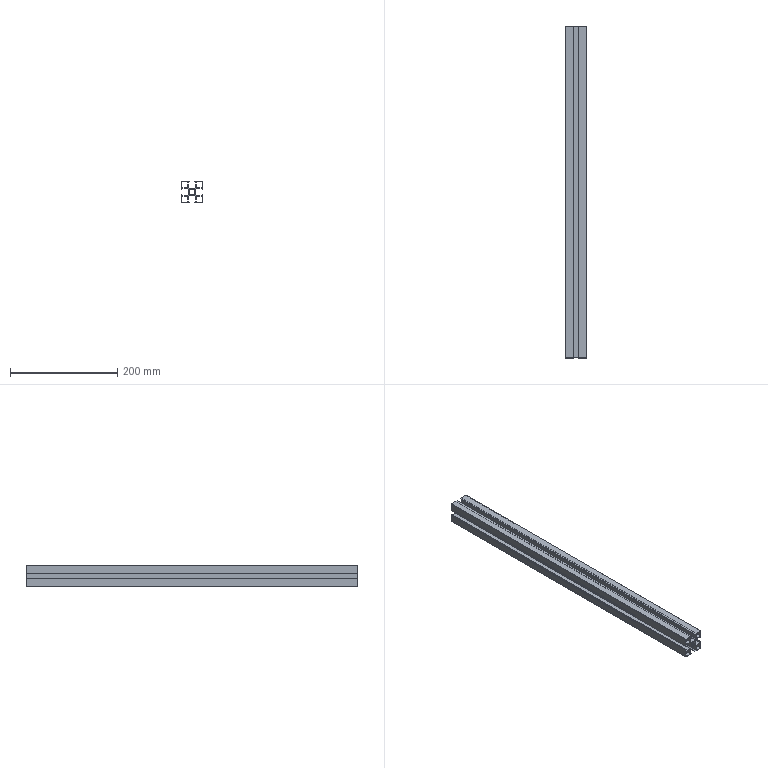Part | SolidWorks | features MirrorPattern 2, Extrusion 1 | 1 solid | 85 faces | box 40 x 620 x 40 mm | volume 161690 mm3 | plane 70 | cylinder 15 | commonest cylinder face diameters 2 x6 10.6 x5 1 x4